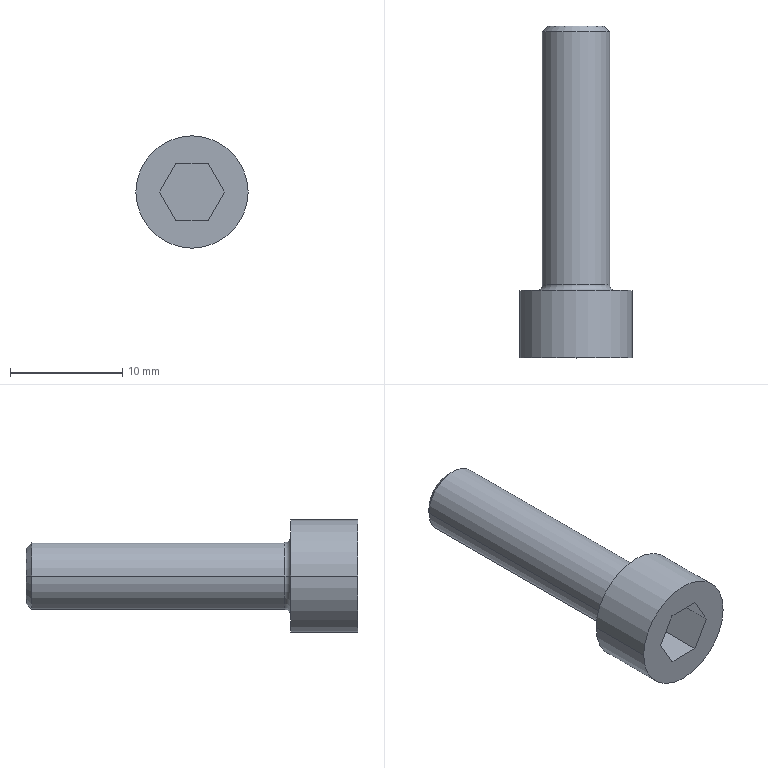Part | STEP file | M6 | 1 solid | 18 faces | box 10 x 29.55 x 10 mm | volume 1049 mm3 | plane 10 | cylinder 4 | torus 2 | cone 2 | commonest cylinder face diameters 6 x2 10 x2
STEP:
#1=CARTESIAN_POINT('',(0.,0.,0.));
#2=DIRECTION('',(0.,0.,1.));
#3=DIRECTION('',(1.,0.,0.));
#4=AXIS2_PLACEMENT_3D('',#1,#2,#3);
#5=CARTESIAN_POINT('',(-3.,6.5,0.));
#6=VERTEX_POINT('',#5);
#7=CARTESIAN_POINT('',(-3.5,6.,0.));
#8=VERTEX_POINT('',#7);
#9=CARTESIAN_POINT('',(-3.5,6.5,0.));
#10=DIRECTION('',(0.,0.,-1.));
#11=DIRECTION('',(-1.,0.,0.));
#12=AXIS2_PLACEMENT_3D('',#9,#10,#11);
#13=CIRCLE('',#12,0.5);
#14=CARTESIAN_POINT('',(0.,6.5,0.));
#15=DIRECTION('',(0.,1.,0.));
#16=DIRECTION('',(-1.,0.,0.));
#17=AXIS2_PLACEMENT_3D('',#14,#15,#16);
#18=TOROIDAL_SURFACE('',#17,3.5,0.5);
#19=CARTESIAN_POINT('',(6.283,0.));
#20=DIRECTION('',(0.,1.));
#21=VECTOR('',#20,1.);
#22=LINE('',#19,#21);
#23=(GEOMETRIC_REPRESENTATION_CONTEXT(2)PARAMETRIC_REPRESENTATION_CONTEXT()REPRESENTATION_CONTEXT('',''));
#24=DEFINITIONAL_REPRESENTATION('',(#22),#23);
#25=PCURVE('',#18,#24);
#26=CARTESIAN_POINT('',(0.,6.5,0.));
#27=DIRECTION('',(0.,1.,0.));
#28=DIRECTION('',(-1.,0.,0.));
#29=AXIS2_PLACEMENT_3D('',#26,#27,#28);
#30=TOROIDAL_SURFACE('',#29,3.5,0.5);
#31=CARTESIAN_POINT('',(0.,0.));
#32=DIRECTION('',(0.,1.));
#33=VECTOR('',#32,1.);
#34=LINE('',#31,#33);
#35=(GEOMETRIC_REPRESENTATION_CONTEXT(2)PARAMETRIC_REPRESENTATION_CONTEXT()REPRESENTATION_CONTEXT('',''));
#36=DEFINITIONAL_REPRESENTATION('',(#34),#35);
#37=PCURVE('',#30,#36);
#38=SURFACE_CURVE('',#13,(#25,#37),.PCURVE_S1.);
#39=EDGE_CURVE('',#6,#8,#38,.T.);
#40=ORIENTED_EDGE('',*,*,#39,.T.);
#41=CARTESIAN_POINT('',(3.5,6.,0.));
#42=VERTEX_POINT('',#41);
#43=CARTESIAN_POINT('',(0.,6.,0.));
#44=DIRECTION('',(0.,-1.,0.));
#45=DIRECTION('',(-1.,0.,0.));
#46=AXIS2_PLACEMENT_3D('',#43,#44,#45);
#47=CIRCLE('',#46,3.5);
#48=CARTESIAN_POINT('',(6.283,4.712));
#49=DIRECTION('',(-1.,0.));
#50=VECTOR('',#49,1.);
#51=LINE('',#48,#50);
#52=(GEOMETRIC_REPRESENTATION_CONTEXT(2)PARAMETRIC_REPRESENTATION_CONTEXT()REPRESENTATION_CONTEXT('',''));
#53=DEFINITIONAL_REPRESENTATION('',(#51),#52);
#54=PCURVE('',#18,#53);
#55=CARTESIAN_POINT('',(5.,6.,0.));
#56=DIRECTION('',(0.,1.,0.));
#57=DIRECTION('',(-1.,0.,0.));
#58=AXIS2_PLACEMENT_3D('',#55,#56,#57);
#59=PLANE('',#58);
#60=CARTESIAN_POINT('',(8.5,0.));
#61=CARTESIAN_POINT('',(8.5,-6.062));
#62=CARTESIAN_POINT('',(3.25,-3.031));
#63=CARTESIAN_POINT('',(-2.,0.));
#64=CARTESIAN_POINT('',(3.25,3.031));
#65=CARTESIAN_POINT('',(8.5,6.062));
#66=CARTESIAN_POINT('',(8.5,0.));
#67=(BOUNDED_CURVE()B_SPLINE_CURVE(2,(#60,#61,#62,#63,#64,#65,#66),.UNSPECIFIED.,.T.,.F.)B_SPLINE_CURVE_WITH_KNOTS((1,2,2,2,2,1),(-2.094,0.,2.094,4.189,6.283,8.378),.UNSPECIFIED.)CURVE()GEOMETRIC_REPRESENTATION_ITEM()RATIONAL_B_SPLINE_CURVE((1.,0.5,1.,0.5,1.,0.5,1.))REPRESENTATION_ITEM(''));
#68=(GEOMETRIC_REPRESENTATION_CONTEXT(2)PARAMETRIC_REPRESENTATION_CONTEXT()REPRESENTATION_CONTEXT('',''));
#69=DEFINITIONAL_REPRESENTATION('',(#67),#68);
#70=PCURVE('',#59,#69);
#71=SURFACE_CURVE('',#47,(#54,#70),.PCURVE_S1.);
#72=EDGE_CURVE('',#8,#42,#71,.T.);
#73=ORIENTED_EDGE('',*,*,#72,.T.);
#74=CARTESIAN_POINT('',(3.,6.5,0.));
#75=VERTEX_POINT('',#74);
#76=CARTESIAN_POINT('',(3.5,6.5,0.));
#77=DIRECTION('',(0.,0.,1.));
#78=DIRECTION('',(1.,0.,0.));
#79=AXIS2_PLACEMENT_3D('',#76,#77,#78);
#80=CIRCLE('',#79,0.5);
#81=CARTESIAN_POINT('',(3.142,0.));
#82=DIRECTION('',(0.,1.));
#83=VECTOR('',#82,1.);
#84=LINE('',#81,#83);
#85=(GEOMETRIC_REPRESENTATION_CONTEXT(2)PARAMETRIC_REPRESENTATION_CONTEXT()REPRESENTATION_CONTEXT('',''));
#86=DEFINITIONAL_REPRESENTATION('',(#84),#85);
#87=PCURVE('',#18,#86);
#88=CARTESIAN_POINT('',(3.142,0.));
#89=DIRECTION('',(0.,1.));
#90=VECTOR('',#89,1.);
#91=LINE('',#88,#90);
#92=(GEOMETRIC_REPRESENTATION_CONTEXT(2)PARAMETRIC_REPRESENTATION_CONTEXT()REPRESENTATION_CONTEXT('',''));
#93=DEFINITIONAL_REPRESENTATION('',(#91),#92);
#94=PCURVE('',#30,#93);
#95=SURFACE_CURVE('',#80,(#87,#94),.PCURVE_S1.);
#96=EDGE_CURVE('',#75,#42,#95,.T.);
#97=ORIENTED_EDGE('',*,*,#96,.F.);
#98=CARTESIAN_POINT('',(0.,6.5,0.));
#99=DIRECTION('',(0.,1.,0.));
#100=DIRECTION('',(-1.,0.,0.));
#101=AXIS2_PLACEMENT_3D('',#98,#99,#100);
#102=CIRCLE('',#101,3.);
#103=CARTESIAN_POINT('',(0.,3.142));
#104=DIRECTION('',(1.,0.));
#105=VECTOR('',#104,1.);
#106=LINE('',#103,#105);
#107=(GEOMETRIC_REPRESENTATION_CONTEXT(2)PARAMETRIC_REPRESENTATION_CONTEXT()REPRESENTATION_CONTEXT('',''));
#108=DEFINITIONAL_REPRESENTATION('',(#106),#107);
#109=PCURVE('',#18,#108);
#110=CARTESIAN_POINT('',(0.,-1000.,0.));
#111=DIRECTION('',(0.,-1.,0.));
#112=DIRECTION('',(1.,0.,0.));
#113=AXIS2_PLACEMENT_3D('',#110,#111,#112);
#114=CYLINDRICAL_SURFACE('',#113,3.);
#115=CARTESIAN_POINT('',(9.425,-1006.5));
#116=DIRECTION('',(-1.,0.));
#117=VECTOR('',#116,1.);
#118=LINE('',#115,#117);
#119=(GEOMETRIC_REPRESENTATION_CONTEXT(2)PARAMETRIC_REPRESENTATION_CONTEXT()REPRESENTATION_CONTEXT('',''));
#120=DEFINITIONAL_REPRESENTATION('',(#118),#119);
#121=PCURVE('',#114,#120);
#122=SURFACE_CURVE('',#102,(#109,#121),.PCURVE_S1.);
#123=EDGE_CURVE('',#75,#6,#122,.T.);
#124=ORIENTED_EDGE('',*,*,#123,.T.);
#125=EDGE_LOOP('',(#40,#73,#97,#124));
#126=FACE_BOUND('',#125,.F.);
#127=ADVANCED_FACE('',(#126),#18,.F.);
#128=CARTESIAN_POINT('',(-2.5,29.55,0.));
#129=VERTEX_POINT('',#128);
#130=CARTESIAN_POINT('',(2.5,29.55,0.));
#131=VERTEX_POINT('',#130);
#132=CARTESIAN_POINT('',(0.,29.55,0.));
#133=DIRECTION('',(0.,1.,0.));
#134=DIRECTION('',(-1.,0.,0.));
#135=AXIS2_PLACEMENT_3D('',#132,#133,#134);
#136=CIRCLE('',#135,2.5);
#137=CARTESIAN_POINT('',(0.,29.05,0.));
#138=DIRECTION('',(0.,-1.,0.));
#139=DIRECTION('',(1.,0.,0.));
#140=AXIS2_PLACEMENT_3D('',#137,#138,#139);
#141=CONICAL_SURFACE('',#140,3.,0.7854);
#142=CARTESIAN_POINT('',(3.142,-0.5));
#143=DIRECTION('',(-1.,0.));
#144=VECTOR('',#143,1.);
#145=LINE('',#142,#144);
#146=(GEOMETRIC_REPRESENTATION_CONTEXT(2)PARAMETRIC_REPRESENTATION_CONTEXT()REPRESENTATION_CONTEXT('',''));
#147=DEFINITIONAL_REPRESENTATION('',(#145),#146);
#148=PCURVE('',#141,#147);
#149=CARTESIAN_POINT('',(3.,29.55,0.));
#150=DIRECTION('',(0.,1.,0.));
#151=DIRECTION('',(-1.,0.,0.));
#152=AXIS2_PLACEMENT_3D('',#149,#150,#151);
#153=PLANE('',#152);
#154=CARTESIAN_POINT('',(3.,0.));
#155=DIRECTION('',(1.,0.));
#156=AXIS2_PLACEMENT_2D('',#154,#155);
#157=CIRCLE('',#156,2.5);
#158=(GEOMETRIC_REPRESENTATION_CONTEXT(2)PARAMETRIC_REPRESENTATION_CONTEXT()REPRESENTATION_CONTEXT('',''));
#159=DEFINITIONAL_REPRESENTATION('',(#157),#158);
#160=PCURVE('',#153,#159);
#161=SURFACE_CURVE('',#136,(#148,#160),.PCURVE_S1.);
#162=EDGE_CURVE('',#129,#131,#161,.T.);
#163=ORIENTED_EDGE('',*,*,#162,.F.);
#164=CARTESIAN_POINT('',(-3.,29.05,0.));
#165=VERTEX_POINT('',#164);
#166=CARTESIAN_POINT('',(-3.,29.05,0.));
#167=DIRECTION('',(-0.7071,-0.7071,0.));
#168=VECTOR('',#167,1.);
#169=LINE('',#166,#168);
#170=CARTESIAN_POINT('',(3.142,0.));
#171=DIRECTION('',(0.,1.));
#172=VECTOR('',#171,1.);
#173=LINE('',#170,#172);
#174=(GEOMETRIC_REPRESENTATION_CONTEXT(2)PARAMETRIC_REPRESENTATION_CONTEXT()REPRESENTATION_CONTEXT('',''));
#175=DEFINITIONAL_REPRESENTATION('',(#173),#174);
#176=PCURVE('',#141,#175);
#177=CARTESIAN_POINT('',(0.,29.05,0.));
#178=DIRECTION('',(0.,-1.,0.));
#179=DIRECTION('',(1.,0.,0.));
#180=AXIS2_PLACEMENT_3D('',#177,#178,#179);
#181=CONICAL_SURFACE('',#180,3.,0.7854);
#182=CARTESIAN_POINT('',(3.142,0.));
#183=DIRECTION('',(0.,1.));
#184=VECTOR('',#183,1.);
#185=LINE('',#182,#184);
#186=(GEOMETRIC_REPRESENTATION_CONTEXT(2)PARAMETRIC_REPRESENTATION_CONTEXT()REPRESENTATION_CONTEXT('',''));
#187=DEFINITIONAL_REPRESENTATION('',(#185),#186);
#188=PCURVE('',#181,#187);
#189=SURFACE_CURVE('',#169,(#176,#188),.PCURVE_S1.);
#190=EDGE_CURVE('',#129,#165,#189,.T.);
#191=ORIENTED_EDGE('',*,*,#190,.T.);
#192=CARTESIAN_POINT('',(3.,29.05,0.));
#193=VERTEX_POINT('',#192);
#194=CARTESIAN_POINT('',(0.,29.05,0.));
#195=DIRECTION('',(0.,-1.,0.));
#196=DIRECTION('',(-1.,0.,0.));
#197=AXIS2_PLACEMENT_3D('',#194,#195,#196);
#198=CIRCLE('',#197,3.);
#199=CARTESIAN_POINT('',(-3.142,0.));
#200=DIRECTION('',(1.,0.));
#201=VECTOR('',#200,1.);
#202=LINE('',#199,#201);
#203=(GEOMETRIC_REPRESENTATION_CONTEXT(2)PARAMETRIC_REPRESENTATION_CONTEXT()REPRESENTATION_CONTEXT('',''));
#204=DEFINITIONAL_REPRESENTATION('',(#202),#203);
#205=PCURVE('',#141,#204);
#206=CARTESIAN_POINT('',(0.,-1000.,0.));
#207=DIRECTION('',(0.,-1.,0.));
#208=DIRECTION('',(1.,0.,0.));
#209=AXIS2_PLACEMENT_3D('',#206,#207,#208);
#210=CYLINDRICAL_SURFACE('',#209,3.);
#211=CARTESIAN_POINT('',(-3.142,-1029.05));
#212=DIRECTION('',(1.,0.));
#213=VECTOR('',#212,1.);
#214=LINE('',#211,#213);
#215=(GEOMETRIC_REPRESENTATION_CONTEXT(2)PARAMETRIC_REPRESENTATION_CONTEXT()REPRESENTATION_CONTEXT('',''));
#216=DEFINITIONAL_REPRESENTATION('',(#214),#215);
#217=PCURVE('',#210,#216);
#218=SURFACE_CURVE('',#198,(#205,#217),.PCURVE_S1.);
#219=EDGE_CURVE('',#193,#165,#218,.T.);
#220=ORIENTED_EDGE('',*,*,#219,.F.);
#221=CARTESIAN_POINT('',(3.,29.05,0.));
#222=DIRECTION('',(0.7071,-0.7071,0.));
#223=VECTOR('',#222,1.);
#224=LINE('',#221,#223);
#225=CARTESIAN_POINT('',(0.,0.));
#226=DIRECTION('',(0.,1.));
#227=VECTOR('',#226,1.);
#228=LINE('',#225,#227);
#229=(GEOMETRIC_REPRESENTATION_CONTEXT(2)PARAMETRIC_REPRESENTATION_CONTEXT()REPRESENTATION_CONTEXT('',''));
#230=DEFINITIONAL_REPRESENTATION('',(#228),#229);
#231=PCURVE('',#141,#230);
#232=CARTESIAN_POINT('',(6.283,0.));
#233=DIRECTION('',(0.,1.));
#234=VECTOR('',#233,1.);
#235=LINE('',#232,#234);
#236=(GEOMETRIC_REPRESENTATION_CONTEXT(2)PARAMETRIC_REPRESENTATION_CONTEXT()REPRESENTATION_CONTEXT('',''));
#237=DEFINITIONAL_REPRESENTATION('',(#235),#236);
#238=PCURVE('',#181,#237);
#239=SURFACE_CURVE('',#224,(#231,#238),.PCURVE_S1.);
#240=EDGE_CURVE('',#131,#193,#239,.T.);
#241=ORIENTED_EDGE('',*,*,#240,.F.);
#242=EDGE_LOOP('',(#163,#191,#220,#241));
#243=FACE_BOUND('',#242,.T.);
#244=ADVANCED_FACE('',(#243),#141,.T.);
#245=ORIENTED_EDGE('',*,*,#219,.T.);
#246=CARTESIAN_POINT('',(-3.,-1000.,0.));
#247=DIRECTION('',(0.,-1.,0.));
#248=VECTOR('',#247,1.);
#249=LINE('',#246,#248);
#250=CARTESIAN_POINT('',(3.142,0.));
#251=DIRECTION('',(0.,1.));
#252=VECTOR('',#251,1.);
#253=LINE('',#250,#252);
#254=(GEOMETRIC_REPRESENTATION_CONTEXT(2)PARAMETRIC_REPRESENTATION_CONTEXT()REPRESENTATION_CONTEXT('',''));
#255=DEFINITIONAL_REPRESENTATION('',(#253),#254);
#256=PCURVE('',#210,#255);
#257=CARTESIAN_POINT('',(3.142,0.));
#258=DIRECTION('',(0.,1.));
#259=VECTOR('',#258,1.);
#260=LINE('',#257,#259);
#261=(GEOMETRIC_REPRESENTATION_CONTEXT(2)PARAMETRIC_REPRESENTATION_CONTEXT()REPRESENTATION_CONTEXT('',''));
#262=DEFINITIONAL_REPRESENTATION('',(#260),#261);
#263=PCURVE('',#114,#262);
#264=SURFACE_CURVE('',#249,(#256,#263),.PCURVE_S1.);
#265=EDGE_CURVE('',#165,#6,#264,.T.);
#266=ORIENTED_EDGE('',*,*,#265,.T.);
#267=CARTESIAN_POINT('',(0.,6.5,0.));
#268=DIRECTION('',(0.,1.,0.));
#269=DIRECTION('',(-1.,0.,0.));
#270=AXIS2_PLACEMENT_3D('',#267,#268,#269);
#271=CIRCLE('',#270,3.);
#272=CARTESIAN_POINT('',(3.142,-1006.5));
#273=DIRECTION('',(-1.,0.));
#274=VECTOR('',#273,1.);
#275=LINE('',#272,#274);
#276=(GEOMETRIC_REPRESENTATION_CONTEXT(2)PARAMETRIC_REPRESENTATION_CONTEXT()REPRESENTATION_CONTEXT('',''));
#277=DEFINITIONAL_REPRESENTATION('',(#275),#276);
#278=PCURVE('',#210,#277);
#279=CARTESIAN_POINT('',(0.,3.142));
#280=DIRECTION('',(1.,0.));
#281=VECTOR('',#280,1.);
#282=LINE('',#279,#281);
#283=(GEOMETRIC_REPRESENTATION_CONTEXT(2)PARAMETRIC_REPRESENTATION_CONTEXT()REPRESENTATION_CONTEXT('',''));
#284=DEFINITIONAL_REPRESENTATION('',(#282),#283);
#285=PCURVE('',#30,#284);
#286=SURFACE_CURVE('',#271,(#278,#285),.PCURVE_S1.);
#287=EDGE_CURVE('',#6,#75,#286,.T.);
#288=ORIENTED_EDGE('',*,*,#287,.T.);
#289=CARTESIAN_POINT('',(3.,-1000.,0.));
#290=DIRECTION('',(0.,-1.,0.));
#291=VECTOR('',#290,1.);
#292=LINE('',#289,#291);
#293=CARTESIAN_POINT('',(0.,0.));
#294=DIRECTION('',(0.,1.));
#295=VECTOR('',#294,1.);
#296=LINE('',#293,#295);
#297=(GEOMETRIC_REPRESENTATION_CONTEXT(2)PARAMETRIC_REPRESENTATION_CONTEXT()REPRESENTATION_CONTEXT('',''));
#298=DEFINITIONAL_REPRESENTATION('',(#296),#297);
#299=PCURVE('',#210,#298);
#300=CARTESIAN_POINT('',(6.283,0.));
#301=DIRECTION('',(0.,1.));
#302=VECTOR('',#301,1.);
#303=LINE('',#300,#302);
#304=(GEOMETRIC_REPRESENTATION_CONTEXT(2)PARAMETRIC_REPRESENTATION_CONTEXT()REPRESENTATION_CONTEXT('',''));
#305=DEFINITIONAL_REPRESENTATION('',(#303),#304);
#306=PCURVE('',#114,#305);
#307=SURFACE_CURVE('',#292,(#299,#306),.PCURVE_S1.);
#308=EDGE_CURVE('',#193,#75,#307,.T.);
#309=ORIENTED_EDGE('',*,*,#308,.F.);
#310=EDGE_LOOP('',(#245,#266,#288,#309));
#311=FACE_BOUND('',#310,.T.);
#312=ADVANCED_FACE('',(#311),#210,.T.);
#313=CARTESIAN_POINT('',(5.,6.,0.));
#314=VERTEX_POINT('',#313);
#315=CARTESIAN_POINT('',(-5.,6.,0.));
#316=VERTEX_POINT('',#315);
#317=CARTESIAN_POINT('',(0.,6.,0.));
#318=DIRECTION('',(0.,-1.,0.));
#319=DIRECTION('',(1.,0.,0.));
#320=AXIS2_PLACEMENT_3D('',#317,#318,#319);
#321=CIRCLE('',#320,5.);
#322=CARTESIAN_POINT('',(0.,-1000.,0.));
#323=DIRECTION('',(0.,-1.,0.));
#324=DIRECTION('',(1.,0.,0.));
#325=AXIS2_PLACEMENT_3D('',#322,#323,#324);
#326=CYLINDRICAL_SURFACE('',#325,5.);
#327=CARTESIAN_POINT('',(0.,-1006.));
#328=DIRECTION('',(1.,0.));
#329=VECTOR('',#328,1.);
#330=LINE('',#327,#329);
#331=(GEOMETRIC_REPRESENTATION_CONTEXT(2)PARAMETRIC_REPRESENTATION_CONTEXT()REPRESENTATION_CONTEXT('',''));
#332=DEFINITIONAL_REPRESENTATION('',(#330),#331);
#333=PCURVE('',#326,#332);
#334=CARTESIAN_POINT('',(0.,0.));
#335=CARTESIAN_POINT('',(0.,8.66));
#336=CARTESIAN_POINT('',(7.5,4.33));
#337=CARTESIAN_POINT('',(15.,0.));
#338=CARTESIAN_POINT('',(7.5,-4.33));
#339=CARTESIAN_POINT('',(0.,-8.66));
#340=CARTESIAN_POINT('',(0.,0.));
#341=(BOUNDED_CURVE()B_SPLINE_CURVE(2,(#334,#335,#336,#337,#338,#339,#340),.UNSPECIFIED.,.T.,.F.)B_SPLINE_CURVE_WITH_KNOTS((1,2,2,2,2,1),(-2.094,0.,2.094,4.189,6.283,8.378),.UNSPECIFIED.)CURVE()GEOMETRIC_REPRESENTATION_ITEM()RATIONAL_B_SPLINE_CURVE((1.,0.5,1.,0.5,1.,0.5,1.))REPRESENTATION_ITEM(''));
#342=(GEOMETRIC_REPRESENTATION_CONTEXT(2)PARAMETRIC_REPRESENTATION_CONTEXT()REPRESENTATION_CONTEXT('',''));
#343=DEFINITIONAL_REPRESENTATION('',(#341),#342);
#344=PCURVE('',#59,#343);
#345=SURFACE_CURVE('',#321,(#333,#344),.PCURVE_S1.);
#346=EDGE_CURVE('',#314,#316,#345,.T.);
#347=ORIENTED_EDGE('',*,*,#346,.T.);
#348=CARTESIAN_POINT('',(-5.,0.,0.));
#349=VERTEX_POINT('',#348);
#350=CARTESIAN_POINT('',(-5.,-1000.,0.));
#351=DIRECTION('',(0.,-1.,0.));
#352=VECTOR('',#351,1.);
#353=LINE('',#350,#352);
#354=CARTESIAN_POINT('',(3.142,0.));
#355=DIRECTION('',(0.,1.));
#356=VECTOR('',#355,1.);
#357=LINE('',#354,#356);
#358=(GEOMETRIC_REPRESENTATION_CONTEXT(2)PARAMETRIC_REPRESENTATION_CONTEXT()REPRESENTATION_CONTEXT('',''));
#359=DEFINITIONAL_REPRESENTATION('',(#357),#358);
#360=PCURVE('',#326,#359);
#361=CARTESIAN_POINT('',(0.,-1000.,0.));
#362=DIRECTION('',(0.,-1.,0.));
#363=DIRECTION('',(1.,0.,0.));
#364=AXIS2_PLACEMENT_3D('',#361,#362,#363);
#365=CYLINDRICAL_SURFACE('',#364,5.);
#366=CARTESIAN_POINT('',(3.142,0.));
#367=DIRECTION('',(0.,1.));
#368=VECTOR('',#367,1.);
#369=LINE('',#366,#368);
#370=(GEOMETRIC_REPRESENTATION_CONTEXT(2)PARAMETRIC_REPRESENTATION_CONTEXT()REPRESENTATION_CONTEXT('',''));
#371=DEFINITIONAL_REPRESENTATION('',(#369),#370);
#372=PCURVE('',#365,#371);
#373=SURFACE_CURVE('',#353,(#360,#372),.PCURVE_S1.);
#374=EDGE_CURVE('',#316,#349,#373,.T.);
#375=ORIENTED_EDGE('',*,*,#374,.T.);
#376=CARTESIAN_POINT('',(5.,0.,0.));
#377=VERTEX_POINT('',#376);
#378=CARTESIAN_POINT('',(0.,0.,0.));
#379=DIRECTION('',(0.,-1.,0.));
#380=DIRECTION('',(1.,0.,0.));
#381=AXIS2_PLACEMENT_3D('',#378,#379,#380);
#382=CIRCLE('',#381,5.);
#383=CARTESIAN_POINT('',(0.,-1000.));
#384=DIRECTION('',(1.,0.));
#385=VECTOR('',#384,1.);
#386=LINE('',#383,#385);
#387=(GEOMETRIC_REPRESENTATION_CONTEXT(2)PARAMETRIC_REPRESENTATION_CONTEXT()REPRESENTATION_CONTEXT('',''));
#388=DEFINITIONAL_REPRESENTATION('',(#386),#387);
#389=PCURVE('',#326,#388);
#390=CARTESIAN_POINT('',(0.,0.,0.));
#391=DIRECTION('',(0.,-1.,0.));
#392=DIRECTION('',(1.,0.,0.));
#393=AXIS2_PLACEMENT_3D('',#390,#391,#392);
#394=PLANE('',#393);
#395=CARTESIAN_POINT('',(0.,0.));
#396=DIRECTION('',(1.,0.));
#397=AXIS2_PLACEMENT_2D('',#395,#396);
#398=CIRCLE('',#397,5.);
#399=(GEOMETRIC_REPRESENTATION_CONTEXT(2)PARAMETRIC_REPRESENTATION_CONTEXT()REPRESENTATION_CONTEXT('',''));
#400=DEFINITIONAL_REPRESENTATION('',(#398),#399);
#401=PCURVE('',#394,#400);
#402=SURFACE_CURVE('',#382,(#389,#401),.PCURVE_S1.);
#403=EDGE_CURVE('',#377,#349,#402,.T.);
#404=ORIENTED_EDGE('',*,*,#403,.F.);
#405=CARTESIAN_POINT('',(5.,-1000.,0.));
#406=DIRECTION('',(0.,-1.,0.));
#407=VECTOR('',#406,1.);
#408=LINE('',#405,#407);
#409=CARTESIAN_POINT('',(0.,0.));
#410=DIRECTION('',(0.,1.));
#411=VECTOR('',#410,1.);
#412=LINE('',#409,#411);
#413=(GEOMETRIC_REPRESENTATION_CONTEXT(2)PARAMETRIC_REPRESENTATION_CONTEXT()REPRESENTATION_CONTEXT('',''));
#414=DEFINITIONAL_REPRESENTATION('',(#412),#413);
#415=PCURVE('',#326,#414);
#416=CARTESIAN_POINT('',(6.283,0.));
#417=DIRECTION('',(0.,1.));
#418=VECTOR('',#417,1.);
#419=LINE('',#416,#418);
#420=(GEOMETRIC_REPRESENTATION_CONTEXT(2)PARAMETRIC_REPRESENTATION_CONTEXT()REPRESENTATION_CONTEXT('',''));
#421=DEFINITIONAL_REPRESENTATION('',(#419),#420);
#422=PCURVE('',#365,#421);
#423=SURFACE_CURVE('',#408,(#415,#422),.PCURVE_S1.);
#424=EDGE_CURVE('',#314,#377,#423,.T.);
#425=ORIENTED_EDGE('',*,*,#424,.F.);
#426=EDGE_LOOP('',(#347,#375,#404,#425));
#427=FACE_BOUND('',#426,.T.);
#428=ADVANCED_FACE('',(#427),#326,.T.);
#429=CARTESIAN_POINT('',(1.443,0.,-2.5));
#430=VERTEX_POINT('',#429);
#431=CARTESIAN_POINT('',(2.887,0.,0.));
#432=VERTEX_POINT('',#431);
#433=CARTESIAN_POINT('',(1.443,0.,-2.5));
#434=DIRECTION('',(0.5,0.,0.866));
#435=VECTOR('',#434,1.);
#436=LINE('',#433,#435);
#437=CARTESIAN_POINT('',(1.443,-2.5));
#438=DIRECTION('',(0.5,0.866));
#439=VECTOR('',#438,1.);
#440=LINE('',#437,#439);
#441=(GEOMETRIC_REPRESENTATION_CONTEXT(2)PARAMETRIC_REPRESENTATION_CONTEXT()REPRESENTATION_CONTEXT('',''));
#442=DEFINITIONAL_REPRESENTATION('',(#440),#441);
#443=PCURVE('',#394,#442);
#444=CARTESIAN_POINT('',(1.443,4.,-2.5));
#445=DIRECTION('',(0.866,0.,-0.5));
#446=DIRECTION('',(-0.5,0.,-0.866));
#447=AXIS2_PLACEMENT_3D('',#444,#445,#446);
#448=PLANE('',#447);
#449=CARTESIAN_POINT('',(0.,-4.));
#450=DIRECTION('',(-1.,0.));
#451=VECTOR('',#450,1.);
#452=LINE('',#449,#451);
#453=(GEOMETRIC_REPRESENTATION_CONTEXT(2)PARAMETRIC_REPRESENTATION_CONTEXT()REPRESENTATION_CONTEXT('',''));
#454=DEFINITIONAL_REPRESENTATION('',(#452),#453);
#455=PCURVE('',#448,#454);
#456=SURFACE_CURVE('',#436,(#443,#455),.PCURVE_S1.);
#457=EDGE_CURVE('',#430,#432,#456,.T.);
#458=ORIENTED_EDGE('',*,*,#457,.F.);
#459=CARTESIAN_POINT('',(-1.443,0.,-2.5));
#460=VERTEX_POINT('',#459);
#461=CARTESIAN_POINT('',(-1.443,0.,-2.5));
#462=DIRECTION('',(1.,0.,0.));
#463=VECTOR('',#462,1.);
#464=LINE('',#461,#463);
#465=CARTESIAN_POINT('',(-1.443,-2.5));
#466=DIRECTION('',(1.,0.));
#467=VECTOR('',#466,1.);
#468=LINE('',#465,#467);
#469=(GEOMETRIC_REPRESENTATION_CONTEXT(2)PARAMETRIC_REPRESENTATION_CONTEXT()REPRESENTATION_CONTEXT('',''));
#470=DEFINITIONAL_REPRESENTATION('',(#468),#469);
#471=PCURVE('',#394,#470);
#472=CARTESIAN_POINT('',(-1.443,4.,-2.5));
#473=DIRECTION('',(0.,0.,-1.));
#474=DIRECTION('',(-1.,0.,0.));
#475=AXIS2_PLACEMENT_3D('',#472,#473,#474);
#476=PLANE('',#475);
#477=CARTESIAN_POINT('',(0.,-4.));
#478=DIRECTION('',(-1.,0.));
#479=VECTOR('',#478,1.);
#480=LINE('',#477,#479);
#481=(GEOMETRIC_REPRESENTATION_CONTEXT(2)PARAMETRIC_REPRESENTATION_CONTEXT()REPRESENTATION_CONTEXT('',''));
#482=DEFINITIONAL_REPRESENTATION('',(#480),#481);
#483=PCURVE('',#476,#482);
#484=SURFACE_CURVE('',#464,(#471,#483),.PCURVE_S1.);
#485=EDGE_CURVE('',#460,#430,#484,.T.);
#486=ORIENTED_EDGE('',*,*,#485,.F.);
#487=CARTESIAN_POINT('',(-2.887,0.,0.));
#488=VERTEX_POINT('',#487);
#489=CARTESIAN_POINT('',(-2.887,0.,0.));
#490=DIRECTION('',(0.5,0.,-0.866));
#491=VECTOR('',#490,1.);
#492=LINE('',#489,#491);
#493=CARTESIAN_POINT('',(-2.887,0.));
#494=DIRECTION('',(0.5,-0.866));
#495=VECTOR('',#494,1.);
#496=LINE('',#493,#495);
#497=(GEOMETRIC_REPRESENTATION_CONTEXT(2)PARAMETRIC_REPRESENTATION_CONTEXT()REPRESENTATION_CONTEXT('',''));
#498=DEFINITIONAL_REPRESENTATION('',(#496),#497);
#499=PCURVE('',#394,#498);
#500=CARTESIAN_POINT('',(-2.887,4.,0.));
#501=DIRECTION('',(-0.866,0.,-0.5));
#502=DIRECTION('',(-0.5,0.,0.866));
#503=AXIS2_PLACEMENT_3D('',#500,#501,#502);
#504=PLANE('',#503);
#505=CARTESIAN_POINT('',(0.,-4.));
#506=DIRECTION('',(-1.,0.));
#507=VECTOR('',#506,1.);
#508=LINE('',#505,#507);
#509=(GEOMETRIC_REPRESENTATION_CONTEXT(2)PARAMETRIC_REPRESENTATION_CONTEXT()REPRESENTATION_CONTEXT('',''));
#510=DEFINITIONAL_REPRESENTATION('',(#508),#509);
#511=PCURVE('',#504,#510);
#512=SURFACE_CURVE('',#492,(#499,#511),.PCURVE_S1.);
#513=EDGE_CURVE('',#488,#460,#512,.T.);
#514=ORIENTED_EDGE('',*,*,#513,.F.);
#515=CARTESIAN_POINT('',(-1.443,0.,2.5));
#516=VERTEX_POINT('',#515);
#517=CARTESIAN_POINT('',(-1.443,0.,2.5));
#518=DIRECTION('',(-0.5,0.,-0.866));
#519=VECTOR('',#518,1.);
#520=LINE('',#517,#519);
#521=CARTESIAN_POINT('',(-1.443,2.5));
#522=DIRECTION('',(-0.5,-0.866));
#523=VECTOR('',#522,1.);
#524=LINE('',#521,#523);
#525=(GEOMETRIC_REPRESENTATION_CONTEXT(2)PARAMETRIC_REPRESENTATION_CONTEXT()REPRESENTATION_CONTEXT('',''));
#526=DEFINITIONAL_REPRESENTATION('',(#524),#525);
#527=PCURVE('',#394,#526);
#528=CARTESIAN_POINT('',(-1.443,4.,2.5));
#529=DIRECTION('',(-0.866,0.,0.5));
#530=DIRECTION('',(0.5,0.,0.866));
#531=AXIS2_PLACEMENT_3D('',#528,#529,#530);
#532=PLANE('',#531);
#533=CARTESIAN_POINT('',(0.,-4.));
#534=DIRECTION('',(-1.,0.));
#535=VECTOR('',#534,1.);
#536=LINE('',#533,#535);
#537=(GEOMETRIC_REPRESENTATION_CONTEXT(2)PARAMETRIC_REPRESENTATION_CONTEXT()REPRESENTATION_CONTEXT('',''));
#538=DEFINITIONAL_REPRESENTATION('',(#536),#537);
#539=PCURVE('',#532,#538);
#540=SURFACE_CURVE('',#520,(#527,#539),.PCURVE_S1.);
#541=EDGE_CURVE('',#516,#488,#540,.T.);
#542=ORIENTED_EDGE('',*,*,#541,.F.);
#543=CARTESIAN_POINT('',(1.443,0.,2.5));
#544=VERTEX_POINT('',#543);
#545=CARTESIAN_POINT('',(1.443,0.,2.5));
#546=DIRECTION('',(-1.,0.,0.));
#547=VECTOR('',#546,1.);
#548=LINE('',#545,#547);
#549=CARTESIAN_POINT('',(1.443,2.5));
#550=DIRECTION('',(-1.,0.));
#551=VECTOR('',#550,1.);
#552=LINE('',#549,#551);
#553=(GEOMETRIC_REPRESENTATION_CONTEXT(2)PARAMETRIC_REPRESENTATION_CONTEXT()REPRESENTATION_CONTEXT('',''));
#554=DEFINITIONAL_REPRESENTATION('',(#552),#553);
#555=PCURVE('',#394,#554);
#556=CARTESIAN_POINT('',(1.443,4.,2.5));
#557=DIRECTION('',(0.,0.,1.));
#558=DIRECTION('',(1.,0.,0.));
#559=AXIS2_PLACEMENT_3D('',#556,#557,#558);
#560=PLANE('',#559);
#561=CARTESIAN_POINT('',(0.,-4.));
#562=DIRECTION('',(-1.,0.));
#563=VECTOR('',#562,1.);
#564=LINE('',#561,#563);
#565=(GEOMETRIC_REPRESENTATION_CONTEXT(2)PARAMETRIC_REPRESENTATION_CONTEXT()REPRESENTATION_CONTEXT('',''));
#566=DEFINITIONAL_REPRESENTATION('',(#564),#565);
#567=PCURVE('',#560,#566);
#568=SURFACE_CURVE('',#548,(#555,#567),.PCURVE_S1.);
#569=EDGE_CURVE('',#544,#516,#568,.T.);
#570=ORIENTED_EDGE('',*,*,#569,.F.);
#571=CARTESIAN_POINT('',(2.887,0.,0.));
#572=DIRECTION('',(-0.5,0.,0.866));
#573=VECTOR('',#572,1.);
#574=LINE('',#571,#573);
#575=CARTESIAN_POINT('',(2.887,0.));
#576=DIRECTION('',(-0.5,0.866));
#577=VECTOR('',#576,1.);
#578=LINE('',#575,#577);
#579=(GEOMETRIC_REPRESENTATION_CONTEXT(2)PARAMETRIC_REPRESENTATION_CONTEXT()REPRESENTATION_CONTEXT('',''));
#580=DEFINITIONAL_REPRESENTATION('',(#578),#579);
#581=PCURVE('',#394,#580);
#582=CARTESIAN_POINT('',(2.887,4.,0.));
#583=DIRECTION('',(0.866,0.,0.5));
#584=DIRECTION('',(0.5,0.,-0.866));
#585=AXIS2_PLACEMENT_3D('',#582,#583,#584);
#586=PLANE('',#585);
#587=CARTESIAN_POINT('',(0.,-4.));
#588=DIRECTION('',(-1.,0.));
#589=VECTOR('',#588,1.);
#590=LINE('',#587,#589);
#591=(GEOMETRIC_REPRESENTATION_CONTEXT(2)PARAMETRIC_REPRESENTATION_CONTEXT()REPRESENTATION_CONTEXT('',''));
#592=DEFINITIONAL_REPRESENTATION('',(#590),#591);
#593=PCURVE('',#586,#592);
#594=SURFACE_CURVE('',#574,(#581,#593),.PCURVE_S1.);
#595=EDGE_CURVE('',#432,#544,#594,.T.);
#596=ORIENTED_EDGE('',*,*,#595,.F.);
#597=EDGE_LOOP('',(#458,#486,#514,#542,#570,#596));
#598=FACE_BOUND('',#597,.T.);
#599=ORIENTED_EDGE('',*,*,#403,.T.);
#600=CARTESIAN_POINT('',(0.,0.,0.));
#601=DIRECTION('',(0.,-1.,0.));
#602=DIRECTION('',(1.,0.,0.));
#603=AXIS2_PLACEMENT_3D('',#600,#601,#602);
#604=CIRCLE('',#603,5.);
#605=CARTESIAN_POINT('',(0.,0.));
#606=DIRECTION('',(1.,0.));
#607=AXIS2_PLACEMENT_2D('',#605,#606);
#608=CIRCLE('',#607,5.);
#609=(GEOMETRIC_REPRESENTATION_CONTEXT(2)PARAMETRIC_REPRESENTATION_CONTEXT()REPRESENTATION_CONTEXT('',''));
#610=DEFINITIONAL_REPRESENTATION('',(#608),#609);
#611=PCURVE('',#394,#610);
#612=CARTESIAN_POINT('',(0.,-1000.));
#613=DIRECTION('',(1.,0.));
#614=VECTOR('',#613,1.);
#615=LINE('',#612,#614);
#616=(GEOMETRIC_REPRESENTATION_CONTEXT(2)PARAMETRIC_REPRESENTATION_CONTEXT()REPRESENTATION_CONTEXT('',''));
#617=DEFINITIONAL_REPRESENTATION('',(#615),#616);
#618=PCURVE('',#365,#617);
#619=SURFACE_CURVE('',#604,(#611,#618),.PCURVE_S1.);
#620=EDGE_CURVE('',#349,#377,#619,.T.);
#621=ORIENTED_EDGE('',*,*,#620,.T.);
#622=EDGE_LOOP('',(#599,#621));
#623=FACE_BOUND('',#622,.T.);
#624=ADVANCED_FACE('',(#598,#623),#394,.T.);
#625=ORIENTED_EDGE('',*,*,#374,.F.);
#626=CARTESIAN_POINT('',(0.,6.,0.));
#627=DIRECTION('',(0.,-1.,0.));
#628=DIRECTION('',(1.,0.,0.));
#629=AXIS2_PLACEMENT_3D('',#626,#627,#628);
#630=CIRCLE('',#629,5.);
#631=CARTESIAN_POINT('',(0.,-1006.));
#632=DIRECTION('',(1.,0.));
#633=VECTOR('',#632,1.);
#634=LINE('',#631,#633);
#635=(GEOMETRIC_REPRESENTATION_CONTEXT(2)PARAMETRIC_REPRESENTATION_CONTEXT()REPRESENTATION_CONTEXT('',''));
#636=DEFINITIONAL_REPRESENTATION('',(#634),#635);
#637=PCURVE('',#365,#636);
#638=CARTESIAN_POINT('',(0.,0.));
#639=CARTESIAN_POINT('',(0.,8.66));
#640=CARTESIAN_POINT('',(7.5,4.33));
#641=CARTESIAN_POINT('',(15.,0.));
#642=CARTESIAN_POINT('',(7.5,-4.33));
#643=CARTESIAN_POINT('',(0.,-8.66));
#644=CARTESIAN_POINT('',(0.,0.));
#645=(BOUNDED_CURVE()B_SPLINE_CURVE(2,(#638,#639,#640,#641,#642,#643,#644),.UNSPECIFIED.,.T.,.F.)B_SPLINE_CURVE_WITH_KNOTS((1,2,2,2,2,1),(-2.094,0.,2.094,4.189,6.283,8.378),.UNSPECIFIED.)CURVE()GEOMETRIC_REPRESENTATION_ITEM()RATIONAL_B_SPLINE_CURVE((1.,0.5,1.,0.5,1.,0.5,1.))REPRESENTATION_ITEM(''));
#646=(GEOMETRIC_REPRESENTATION_CONTEXT(2)PARAMETRIC_REPRESENTATION_CONTEXT()REPRESENTATION_CONTEXT('',''));
#647=DEFINITIONAL_REPRESENTATION('',(#645),#646);
#648=PCURVE('',#59,#647);
#649=SURFACE_CURVE('',#630,(#637,#648),.PCURVE_S1.);
#650=EDGE_CURVE('',#316,#314,#649,.T.);
#651=ORIENTED_EDGE('',*,*,#650,.T.);
#652=ORIENTED_EDGE('',*,*,#424,.T.);
#653=ORIENTED_EDGE('',*,*,#620,.F.);
#654=EDGE_LOOP('',(#625,#651,#652,#653));
#655=FACE_BOUND('',#654,.T.);
#656=ADVANCED_FACE('',(#655),#365,.T.);
#657=ORIENTED_EDGE('',*,*,#72,.T.);
#658=CARTESIAN_POINT('',(0.,6.,0.));
#659=DIRECTION('',(0.,-1.,0.));
#660=DIRECTION('',(-1.,0.,0.));
#661=AXIS2_PLACEMENT_3D('',#658,#659,#660);
#662=CIRCLE('',#661,3.5);
#663=CARTESIAN_POINT('',(8.5,0.));
#664=CARTESIAN_POINT('',(8.5,-6.062));
#665=CARTESIAN_POINT('',(3.25,-3.031));
#666=CARTESIAN_POINT('',(-2.,0.));
#667=CARTESIAN_POINT('',(3.25,3.031));
#668=CARTESIAN_POINT('',(8.5,6.062));
#669=CARTESIAN_POINT('',(8.5,0.));
#670=(BOUNDED_CURVE()B_SPLINE_CURVE(2,(#663,#664,#665,#666,#667,#668,#669),.UNSPECIFIED.,.T.,.F.)B_SPLINE_CURVE_WITH_KNOTS((1,2,2,2,2,1),(-2.094,0.,2.094,4.189,6.283,8.378),.UNSPECIFIED.)CURVE()GEOMETRIC_REPRESENTATION_ITEM()RATIONAL_B_SPLINE_CURVE((1.,0.5,1.,0.5,1.,0.5,1.))REPRESENTATION_ITEM(''));
#671=(GEOMETRIC_REPRESENTATION_CONTEXT(2)PARAMETRIC_REPRESENTATION_CONTEXT()REPRESENTATION_CONTEXT('',''));
#672=DEFINITIONAL_REPRESENTATION('',(#670),#671);
#673=PCURVE('',#59,#672);
#674=CARTESIAN_POINT('',(6.283,4.712));
#675=DIRECTION('',(-1.,0.));
#676=VECTOR('',#675,1.);
#677=LINE('',#674,#676);
#678=(GEOMETRIC_REPRESENTATION_CONTEXT(2)PARAMETRIC_REPRESENTATION_CONTEXT()REPRESENTATION_CONTEXT('',''));
#679=DEFINITIONAL_REPRESENTATION('',(#677),#678);
#680=PCURVE('',#30,#679);
#681=SURFACE_CURVE('',#662,(#673,#680),.PCURVE_S1.);
#682=EDGE_CURVE('',#42,#8,#681,.T.);
#683=ORIENTED_EDGE('',*,*,#682,.T.);
#684=EDGE_LOOP('',(#657,#683));
#685=FACE_BOUND('',#684,.T.);
#686=ORIENTED_EDGE('',*,*,#346,.F.);
#687=ORIENTED_EDGE('',*,*,#650,.F.);
#688=EDGE_LOOP('',(#686,#687));
#689=FACE_BOUND('',#688,.T.);
#690=ADVANCED_FACE('',(#685,#689),#59,.T.);
#691=ORIENTED_EDGE('',*,*,#265,.F.);
#692=CARTESIAN_POINT('',(0.,29.05,0.));
#693=DIRECTION('',(0.,-1.,0.));
#694=DIRECTION('',(-1.,0.,0.));
#695=AXIS2_PLACEMENT_3D('',#692,#693,#694);
#696=CIRCLE('',#695,3.);
#697=CARTESIAN_POINT('',(3.142,-1029.05));
#698=DIRECTION('',(1.,0.));
#699=VECTOR('',#698,1.);
#700=LINE('',#697,#699);
#701=(GEOMETRIC_REPRESENTATION_CONTEXT(2)PARAMETRIC_REPRESENTATION_CONTEXT()REPRESENTATION_CONTEXT('',''));
#702=DEFINITIONAL_REPRESENTATION('',(#700),#701);
#703=PCURVE('',#114,#702);
#704=CARTESIAN_POINT('',(3.142,0.));
#705=DIRECTION('',(1.,0.));
#706=VECTOR('',#705,1.);
#707=LINE('',#704,#706);
#708=(GEOMETRIC_REPRESENTATION_CONTEXT(2)PARAMETRIC_REPRESENTATION_CONTEXT()REPRESENTATION_CONTEXT('',''));
#709=DEFINITIONAL_REPRESENTATION('',(#707),#708);
#710=PCURVE('',#181,#709);
#711=SURFACE_CURVE('',#696,(#703,#710),.PCURVE_S1.);
#712=EDGE_CURVE('',#165,#193,#711,.T.);
#713=ORIENTED_EDGE('',*,*,#712,.T.);
#714=ORIENTED_EDGE('',*,*,#308,.T.);
#715=ORIENTED_EDGE('',*,*,#123,.T.);
#716=EDGE_LOOP('',(#691,#713,#714,#715));
#717=FACE_BOUND('',#716,.T.);
#718=ADVANCED_FACE('',(#717),#114,.T.);
#719=CARTESIAN_POINT('',(0.,29.55,0.));
#720=DIRECTION('',(0.,1.,0.));
#721=DIRECTION('',(-1.,0.,0.));
#722=AXIS2_PLACEMENT_3D('',#719,#720,#721);
#723=CIRCLE('',#722,2.5);
#724=CARTESIAN_POINT('',(3.,0.));
#725=DIRECTION('',(1.,0.));
#726=AXIS2_PLACEMENT_2D('',#724,#725);
#727=CIRCLE('',#726,2.5);
#728=(GEOMETRIC_REPRESENTATION_CONTEXT(2)PARAMETRIC_REPRESENTATION_CONTEXT()REPRESENTATION_CONTEXT('',''));
#729=DEFINITIONAL_REPRESENTATION('',(#727),#728);
#730=PCURVE('',#153,#729);
#731=CARTESIAN_POINT('',(9.425,-0.5));
#732=DIRECTION('',(-1.,0.));
#733=VECTOR('',#732,1.);
#734=LINE('',#731,#733);
#735=(GEOMETRIC_REPRESENTATION_CONTEXT(2)PARAMETRIC_REPRESENTATION_CONTEXT()REPRESENTATION_CONTEXT('',''));
#736=DEFINITIONAL_REPRESENTATION('',(#734),#735);
#737=PCURVE('',#181,#736);
#738=SURFACE_CURVE('',#723,(#730,#737),.PCURVE_S1.);
#739=EDGE_CURVE('',#131,#129,#738,.T.);
#740=ORIENTED_EDGE('',*,*,#739,.T.);
#741=ORIENTED_EDGE('',*,*,#162,.T.);
#742=EDGE_LOOP('',(#740,#741));
#743=FACE_BOUND('',#742,.T.);
#744=ADVANCED_FACE('',(#743),#153,.T.);
#745=ORIENTED_EDGE('',*,*,#457,.T.);
#746=CARTESIAN_POINT('',(2.887,4.,0.));
#747=VERTEX_POINT('',#746);
#748=CARTESIAN_POINT('',(2.887,4.,0.));
#749=DIRECTION('',(0.,-1.,0.));
#750=VECTOR('',#749,1.);
#751=LINE('',#748,#750);
#752=CARTESIAN_POINT('',(-2.887,0.));
#753=DIRECTION('',(0.,-1.));
#754=VECTOR('',#753,1.);
#755=LINE('',#752,#754);
#756=(GEOMETRIC_REPRESENTATION_CONTEXT(2)PARAMETRIC_REPRESENTATION_CONTEXT()REPRESENTATION_CONTEXT('',''));
#757=DEFINITIONAL_REPRESENTATION('',(#755),#756);
#758=PCURVE('',#448,#757);
#759=CARTESIAN_POINT('',(0.,0.));
#760=DIRECTION('',(0.,-1.));
#761=VECTOR('',#760,1.);
#762=LINE('',#759,#761);
#763=(GEOMETRIC_REPRESENTATION_CONTEXT(2)PARAMETRIC_REPRESENTATION_CONTEXT()REPRESENTATION_CONTEXT('',''));
#764=DEFINITIONAL_REPRESENTATION('',(#762),#763);
#765=PCURVE('',#586,#764);
#766=SURFACE_CURVE('',#751,(#758,#765),.PCURVE_S1.);
#767=EDGE_CURVE('',#747,#432,#766,.T.);
#768=ORIENTED_EDGE('',*,*,#767,.F.);
#769=CARTESIAN_POINT('',(1.443,4.,-2.5));
#770=VERTEX_POINT('',#769);
#771=CARTESIAN_POINT('',(1.443,4.,-2.5));
#772=DIRECTION('',(0.5,0.,0.866));
#773=VECTOR('',#772,1.);
#774=LINE('',#771,#773);
#775=CARTESIAN_POINT('',(0.,0.));
#776=DIRECTION('',(-1.,0.));
#777=VECTOR('',#776,1.);
#778=LINE('',#775,#777);
#779=(GEOMETRIC_REPRESENTATION_CONTEXT(2)PARAMETRIC_REPRESENTATION_CONTEXT()REPRESENTATION_CONTEXT('',''));
#780=DEFINITIONAL_REPRESENTATION('',(#778),#779);
#781=PCURVE('',#448,#780);
#782=CARTESIAN_POINT('',(1.443,4.,-2.5));
#783=DIRECTION('',(0.,1.,0.));
#784=DIRECTION('',(-1.,0.,0.));
#785=AXIS2_PLACEMENT_3D('',#782,#783,#784);
#786=PLANE('',#785);
#787=CARTESIAN_POINT('',(0.,0.));
#788=DIRECTION('',(-0.5,0.866));
#789=VECTOR('',#788,1.);
#790=LINE('',#787,#789);
#791=(GEOMETRIC_REPRESENTATION_CONTEXT(2)PARAMETRIC_REPRESENTATION_CONTEXT()REPRESENTATION_CONTEXT('',''));
#792=DEFINITIONAL_REPRESENTATION('',(#790),#791);
#793=PCURVE('',#786,#792);
#794=SURFACE_CURVE('',#774,(#781,#793),.PCURVE_S1.);
#795=EDGE_CURVE('',#770,#747,#794,.T.);
#796=ORIENTED_EDGE('',*,*,#795,.F.);
#797=CARTESIAN_POINT('',(1.443,4.,-2.5));
#798=DIRECTION('',(0.,-1.,0.));
#799=VECTOR('',#798,1.);
#800=LINE('',#797,#799);
#801=CARTESIAN_POINT('',(0.,0.));
#802=DIRECTION('',(0.,-1.));
#803=VECTOR('',#802,1.);
#804=LINE('',#801,#803);
#805=(GEOMETRIC_REPRESENTATION_CONTEXT(2)PARAMETRIC_REPRESENTATION_CONTEXT()REPRESENTATION_CONTEXT('',''));
#806=DEFINITIONAL_REPRESENTATION('',(#804),#805);
#807=PCURVE('',#448,#806);
#808=CARTESIAN_POINT('',(-2.887,0.));
#809=DIRECTION('',(0.,-1.));
#810=VECTOR('',#809,1.);
#811=LINE('',#808,#810);
#812=(GEOMETRIC_REPRESENTATION_CONTEXT(2)PARAMETRIC_REPRESENTATION_CONTEXT()REPRESENTATION_CONTEXT('',''));
#813=DEFINITIONAL_REPRESENTATION('',(#811),#812);
#814=PCURVE('',#476,#813);
#815=SURFACE_CURVE('',#800,(#807,#814),.PCURVE_S1.);
#816=EDGE_CURVE('',#770,#430,#815,.T.);
#817=ORIENTED_EDGE('',*,*,#816,.T.);
#818=EDGE_LOOP('',(#745,#768,#796,#817));
#819=FACE_BOUND('',#818,.T.);
#820=ADVANCED_FACE('',(#819),#448,.F.);
#821=ORIENTED_EDGE('',*,*,#485,.T.);
#822=ORIENTED_EDGE('',*,*,#816,.F.);
#823=CARTESIAN_POINT('',(-1.443,4.,-2.5));
#824=VERTEX_POINT('',#823);
#825=CARTESIAN_POINT('',(-1.443,4.,-2.5));
#826=DIRECTION('',(1.,0.,0.));
#827=VECTOR('',#826,1.);
#828=LINE('',#825,#827);
#829=CARTESIAN_POINT('',(0.,0.));
#830=DIRECTION('',(-1.,0.));
#831=VECTOR('',#830,1.);
#832=LINE('',#829,#831);
#833=(GEOMETRIC_REPRESENTATION_CONTEXT(2)PARAMETRIC_REPRESENTATION_CONTEXT()REPRESENTATION_CONTEXT('',''));
#834=DEFINITIONAL_REPRESENTATION('',(#832),#833);
#835=PCURVE('',#476,#834);
#836=CARTESIAN_POINT('',(2.887,0.));
#837=DIRECTION('',(-1.,0.));
#838=VECTOR('',#837,1.);
#839=LINE('',#836,#838);
#840=(GEOMETRIC_REPRESENTATION_CONTEXT(2)PARAMETRIC_REPRESENTATION_CONTEXT()REPRESENTATION_CONTEXT('',''));
#841=DEFINITIONAL_REPRESENTATION('',(#839),#840);
#842=PCURVE('',#786,#841);
#843=SURFACE_CURVE('',#828,(#835,#842),.PCURVE_S1.);
#844=EDGE_CURVE('',#824,#770,#843,.T.);
#845=ORIENTED_EDGE('',*,*,#844,.F.);
#846=CARTESIAN_POINT('',(-1.443,4.,-2.5));
#847=DIRECTION('',(0.,-1.,0.));
#848=VECTOR('',#847,1.);
#849=LINE('',#846,#848);
#850=CARTESIAN_POINT('',(0.,0.));
#851=DIRECTION('',(0.,-1.));
#852=VECTOR('',#851,1.);
#853=LINE('',#850,#852);
#854=(GEOMETRIC_REPRESENTATION_CONTEXT(2)PARAMETRIC_REPRESENTATION_CONTEXT()REPRESENTATION_CONTEXT('',''));
#855=DEFINITIONAL_REPRESENTATION('',(#853),#854);
#856=PCURVE('',#476,#855);
#857=CARTESIAN_POINT('',(-2.887,0.));
#858=DIRECTION('',(0.,-1.));
#859=VECTOR('',#858,1.);
#860=LINE('',#857,#859);
#861=(GEOMETRIC_REPRESENTATION_CONTEXT(2)PARAMETRIC_REPRESENTATION_CONTEXT()REPRESENTATION_CONTEXT('',''));
#862=DEFINITIONAL_REPRESENTATION('',(#860),#861);
#863=PCURVE('',#504,#862);
#864=SURFACE_CURVE('',#849,(#856,#863),.PCURVE_S1.);
#865=EDGE_CURVE('',#824,#460,#864,.T.);
#866=ORIENTED_EDGE('',*,*,#865,.T.);
#867=EDGE_LOOP('',(#821,#822,#845,#866));
#868=FACE_BOUND('',#867,.T.);
#869=ADVANCED_FACE('',(#868),#476,.F.);
#870=ORIENTED_EDGE('',*,*,#513,.T.);
#871=ORIENTED_EDGE('',*,*,#865,.F.);
#872=CARTESIAN_POINT('',(-2.887,4.,0.));
#873=VERTEX_POINT('',#872);
#874=CARTESIAN_POINT('',(-2.887,4.,0.));
#875=DIRECTION('',(0.5,0.,-0.866));
#876=VECTOR('',#875,1.);
#877=LINE('',#874,#876);
#878=CARTESIAN_POINT('',(0.,0.));
#879=DIRECTION('',(-1.,0.));
#880=VECTOR('',#879,1.);
#881=LINE('',#878,#880);
#882=(GEOMETRIC_REPRESENTATION_CONTEXT(2)PARAMETRIC_REPRESENTATION_CONTEXT()REPRESENTATION_CONTEXT('',''));
#883=DEFINITIONAL_REPRESENTATION('',(#881),#882);
#884=PCURVE('',#504,#883);
#885=CARTESIAN_POINT('',(4.33,2.5));
#886=DIRECTION('',(-0.5,-0.866));
#887=VECTOR('',#886,1.);
#888=LINE('',#885,#887);
#889=(GEOMETRIC_REPRESENTATION_CONTEXT(2)PARAMETRIC_REPRESENTATION_CONTEXT()REPRESENTATION_CONTEXT('',''));
#890=DEFINITIONAL_REPRESENTATION('',(#888),#889);
#891=PCURVE('',#786,#890);
#892=SURFACE_CURVE('',#877,(#884,#891),.PCURVE_S1.);
#893=EDGE_CURVE('',#873,#824,#892,.T.);
#894=ORIENTED_EDGE('',*,*,#893,.F.);
#895=CARTESIAN_POINT('',(-2.887,4.,0.));
#896=DIRECTION('',(0.,-1.,0.));
#897=VECTOR('',#896,1.);
#898=LINE('',#895,#897);
#899=CARTESIAN_POINT('',(0.,0.));
#900=DIRECTION('',(0.,-1.));
#901=VECTOR('',#900,1.);
#902=LINE('',#899,#901);
#903=(GEOMETRIC_REPRESENTATION_CONTEXT(2)PARAMETRIC_REPRESENTATION_CONTEXT()REPRESENTATION_CONTEXT('',''));
#904=DEFINITIONAL_REPRESENTATION('',(#902),#903);
#905=PCURVE('',#504,#904);
#906=CARTESIAN_POINT('',(-2.887,0.));
#907=DIRECTION('',(0.,-1.));
#908=VECTOR('',#907,1.);
#909=LINE('',#906,#908);
#910=(GEOMETRIC_REPRESENTATION_CONTEXT(2)PARAMETRIC_REPRESENTATION_CONTEXT()REPRESENTATION_CONTEXT('',''));
#911=DEFINITIONAL_REPRESENTATION('',(#909),#910);
#912=PCURVE('',#532,#911);
#913=SURFACE_CURVE('',#898,(#905,#912),.PCURVE_S1.);
#914=EDGE_CURVE('',#873,#488,#913,.T.);
#915=ORIENTED_EDGE('',*,*,#914,.T.);
#916=EDGE_LOOP('',(#870,#871,#894,#915));
#917=FACE_BOUND('',#916,.T.);
#918=ADVANCED_FACE('',(#917),#504,.F.);
#919=ORIENTED_EDGE('',*,*,#541,.T.);
#920=ORIENTED_EDGE('',*,*,#914,.F.);
#921=CARTESIAN_POINT('',(-1.443,4.,2.5));
#922=VERTEX_POINT('',#921);
#923=CARTESIAN_POINT('',(-1.443,4.,2.5));
#924=DIRECTION('',(-0.5,0.,-0.866));
#925=VECTOR('',#924,1.);
#926=LINE('',#923,#925);
#927=CARTESIAN_POINT('',(0.,0.));
#928=DIRECTION('',(-1.,0.));
#929=VECTOR('',#928,1.);
#930=LINE('',#927,#929);
#931=(GEOMETRIC_REPRESENTATION_CONTEXT(2)PARAMETRIC_REPRESENTATION_CONTEXT()REPRESENTATION_CONTEXT('',''));
#932=DEFINITIONAL_REPRESENTATION('',(#930),#931);
#933=PCURVE('',#532,#932);
#934=CARTESIAN_POINT('',(2.887,5.));
#935=DIRECTION('',(0.5,-0.866));
#936=VECTOR('',#935,1.);
#937=LINE('',#934,#936);
#938=(GEOMETRIC_REPRESENTATION_CONTEXT(2)PARAMETRIC_REPRESENTATION_CONTEXT()REPRESENTATION_CONTEXT('',''));
#939=DEFINITIONAL_REPRESENTATION('',(#937),#938);
#940=PCURVE('',#786,#939);
#941=SURFACE_CURVE('',#926,(#933,#940),.PCURVE_S1.);
#942=EDGE_CURVE('',#922,#873,#941,.T.);
#943=ORIENTED_EDGE('',*,*,#942,.F.);
#944=CARTESIAN_POINT('',(-1.443,4.,2.5));
#945=DIRECTION('',(0.,-1.,0.));
#946=VECTOR('',#945,1.);
#947=LINE('',#944,#946);
#948=CARTESIAN_POINT('',(0.,0.));
#949=DIRECTION('',(0.,-1.));
#950=VECTOR('',#949,1.);
#951=LINE('',#948,#950);
#952=(GEOMETRIC_REPRESENTATION_CONTEXT(2)PARAMETRIC_REPRESENTATION_CONTEXT()REPRESENTATION_CONTEXT('',''));
#953=DEFINITIONAL_REPRESENTATION('',(#951),#952);
#954=PCURVE('',#532,#953);
#955=CARTESIAN_POINT('',(-2.887,0.));
#956=DIRECTION('',(0.,-1.));
#957=VECTOR('',#956,1.);
#958=LINE('',#955,#957);
#959=(GEOMETRIC_REPRESENTATION_CONTEXT(2)PARAMETRIC_REPRESENTATION_CONTEXT()REPRESENTATION_CONTEXT('',''));
#960=DEFINITIONAL_REPRESENTATION('',(#958),#959);
#961=PCURVE('',#560,#960);
#962=SURFACE_CURVE('',#947,(#954,#961),.PCURVE_S1.);
#963=EDGE_CURVE('',#922,#516,#962,.T.);
#964=ORIENTED_EDGE('',*,*,#963,.T.);
#965=EDGE_LOOP('',(#919,#920,#943,#964));
#966=FACE_BOUND('',#965,.T.);
#967=ADVANCED_FACE('',(#966),#532,.F.);
#968=ORIENTED_EDGE('',*,*,#569,.T.);
#969=ORIENTED_EDGE('',*,*,#963,.F.);
#970=CARTESIAN_POINT('',(1.443,4.,2.5));
#971=VERTEX_POINT('',#970);
#972=CARTESIAN_POINT('',(1.443,4.,2.5));
#973=DIRECTION('',(-1.,0.,0.));
#974=VECTOR('',#973,1.);
#975=LINE('',#972,#974);
#976=CARTESIAN_POINT('',(0.,0.));
#977=DIRECTION('',(-1.,0.));
#978=VECTOR('',#977,1.);
#979=LINE('',#976,#978);
#980=(GEOMETRIC_REPRESENTATION_CONTEXT(2)PARAMETRIC_REPRESENTATION_CONTEXT()REPRESENTATION_CONTEXT('',''));
#981=DEFINITIONAL_REPRESENTATION('',(#979),#980);
#982=PCURVE('',#560,#981);
#983=CARTESIAN_POINT('',(0.,5.));
#984=DIRECTION('',(1.,0.));
#985=VECTOR('',#984,1.);
#986=LINE('',#983,#985);
#987=(GEOMETRIC_REPRESENTATION_CONTEXT(2)PARAMETRIC_REPRESENTATION_CONTEXT()REPRESENTATION_CONTEXT('',''));
#988=DEFINITIONAL_REPRESENTATION('',(#986),#987);
#989=PCURVE('',#786,#988);
#990=SURFACE_CURVE('',#975,(#982,#989),.PCURVE_S1.);
#991=EDGE_CURVE('',#971,#922,#990,.T.);
#992=ORIENTED_EDGE('',*,*,#991,.F.);
#993=CARTESIAN_POINT('',(1.443,4.,2.5));
#994=DIRECTION('',(0.,-1.,0.));
#995=VECTOR('',#994,1.);
#996=LINE('',#993,#995);
#997=CARTESIAN_POINT('',(0.,0.));
#998=DIRECTION('',(0.,-1.));
#999=VECTOR('',#998,1.);
#1000=LINE('',#997,#999);
#1001=(GEOMETRIC_REPRESENTATION_CONTEXT(2)PARAMETRIC_REPRESENTATION_CONTEXT()REPRESENTATION_CONTEXT('',''));
#1002=DEFINITIONAL_REPRESENTATION('',(#1000),#1001);
#1003=PCURVE('',#560,#1002);
#1004=CARTESIAN_POINT('',(-2.887,0.));
#1005=DIRECTION('',(0.,-1.));
#1006=VECTOR('',#1005,1.);
#1007=LINE('',#1004,#1006);
#1008=(GEOMETRIC_REPRESENTATION_CONTEXT(2)PARAMETRIC_REPRESENTATION_CONTEXT()REPRESENTATION_CONTEXT('',''));
#1009=DEFINITIONAL_REPRESENTATION('',(#1007),#1008);
#1010=PCURVE('',#586,#1009);
#1011=SURFACE_CURVE('',#996,(#1003,#1010),.PCURVE_S1.);
#1012=EDGE_CURVE('',#971,#544,#1011,.T.);
#1013=ORIENTED_EDGE('',*,*,#1012,.T.);
#1014=EDGE_LOOP('',(#968,#969,#992,#1013));
#1015=FACE_BOUND('',#1014,.T.);
#1016=ADVANCED_FACE('',(#1015),#560,.F.);
#1017=ORIENTED_EDGE('',*,*,#595,.T.);
#1018=ORIENTED_EDGE('',*,*,#1012,.F.);
#1019=CARTESIAN_POINT('',(2.887,4.,0.));
#1020=DIRECTION('',(-0.5,0.,0.866));
#1021=VECTOR('',#1020,1.);
#1022=LINE('',#1019,#1021);
#1023=CARTESIAN_POINT('',(0.,0.));
#1024=DIRECTION('',(-1.,0.));
#1025=VECTOR('',#1024,1.);
#1026=LINE('',#1023,#1025);
#1027=(GEOMETRIC_REPRESENTATION_CONTEXT(2)PARAMETRIC_REPRESENTATION_CONTEXT()REPRESENTATION_CONTEXT('',''));
#1028=DEFINITIONAL_REPRESENTATION('',(#1026),#1027);
#1029=PCURVE('',#586,#1028);
#1030=CARTESIAN_POINT('',(-1.443,2.5));
#1031=DIRECTION('',(0.5,0.866));
#1032=VECTOR('',#1031,1.);
#1033=LINE('',#1030,#1032);
#1034=(GEOMETRIC_REPRESENTATION_CONTEXT(2)PARAMETRIC_REPRESENTATION_CONTEXT()REPRESENTATION_CONTEXT('',''));
#1035=DEFINITIONAL_REPRESENTATION('',(#1033),#1034);
#1036=PCURVE('',#786,#1035);
#1037=SURFACE_CURVE('',#1022,(#1029,#1036),.PCURVE_S1.);
#1038=EDGE_CURVE('',#747,#971,#1037,.T.);
#1039=ORIENTED_EDGE('',*,*,#1038,.F.);
#1040=ORIENTED_EDGE('',*,*,#767,.T.);
#1041=EDGE_LOOP('',(#1017,#1018,#1039,#1040));
#1042=FACE_BOUND('',#1041,.T.);
#1043=ADVANCED_FACE('',(#1042),#586,.F.);
#1044=ORIENTED_EDGE('',*,*,#795,.T.);
#1045=ORIENTED_EDGE('',*,*,#1038,.T.);
#1046=ORIENTED_EDGE('',*,*,#991,.T.);
#1047=ORIENTED_EDGE('',*,*,#942,.T.);
#1048=ORIENTED_EDGE('',*,*,#893,.T.);
#1049=ORIENTED_EDGE('',*,*,#844,.T.);
#1050=EDGE_LOOP('',(#1044,#1045,#1046,#1047,#1048,#1049));
#1051=FACE_BOUND('',#1050,.T.);
#1052=ADVANCED_FACE('',(#1051),#786,.F.);
#1053=ORIENTED_EDGE('',*,*,#190,.F.);
#1054=ORIENTED_EDGE('',*,*,#739,.F.);
#1055=ORIENTED_EDGE('',*,*,#240,.T.);
#1056=ORIENTED_EDGE('',*,*,#712,.F.);
#1057=EDGE_LOOP('',(#1053,#1054,#1055,#1056));
#1058=FACE_BOUND('',#1057,.T.);
#1059=ADVANCED_FACE('',(#1058),#181,.T.);
#1060=ORIENTED_EDGE('',*,*,#682,.T.);
#1061=ORIENTED_EDGE('',*,*,#39,.F.);
#1062=ORIENTED_EDGE('',*,*,#287,.T.);
#1063=ORIENTED_EDGE('',*,*,#96,.T.);
#1064=EDGE_LOOP('',(#1060,#1061,#1062,#1063));
#1065=FACE_BOUND('',#1064,.F.);
#1066=ADVANCED_FACE('',(#1065),#30,.F.);
#1067=CLOSED_SHELL('',(#127,#244,#312,#428,#624,#656,#690,#718,#744,#820,#869,#918,#967,#1016,#1043,#1052,#1059,#1066));
#1068=MANIFOLD_SOLID_BREP('',#1067);
#1069=(LENGTH_UNIT()NAMED_UNIT(*)SI_UNIT(.MILLI.,.METRE.));
#1070=UNCERTAINTY_MEASURE_WITH_UNIT(LENGTH_MEASURE(0.0000001),#1069,'','');
#1071=(NAMED_UNIT(*)PLANE_ANGLE_UNIT()SI_UNIT($,.RADIAN.));
#1072=(NAMED_UNIT(*)SI_UNIT($,.STERADIAN.)SOLID_ANGLE_UNIT());
#1073=(GEOMETRIC_REPRESENTATION_CONTEXT(3)GLOBAL_UNCERTAINTY_ASSIGNED_CONTEXT((#1070))GLOBAL_UNIT_ASSIGNED_CONTEXT((#1069,#1071,#1072))REPRESENTATION_CONTEXT('',''));
#1074=ADVANCED_BREP_SHAPE_REPRESENTATION('',(#4,#1068),#1073);